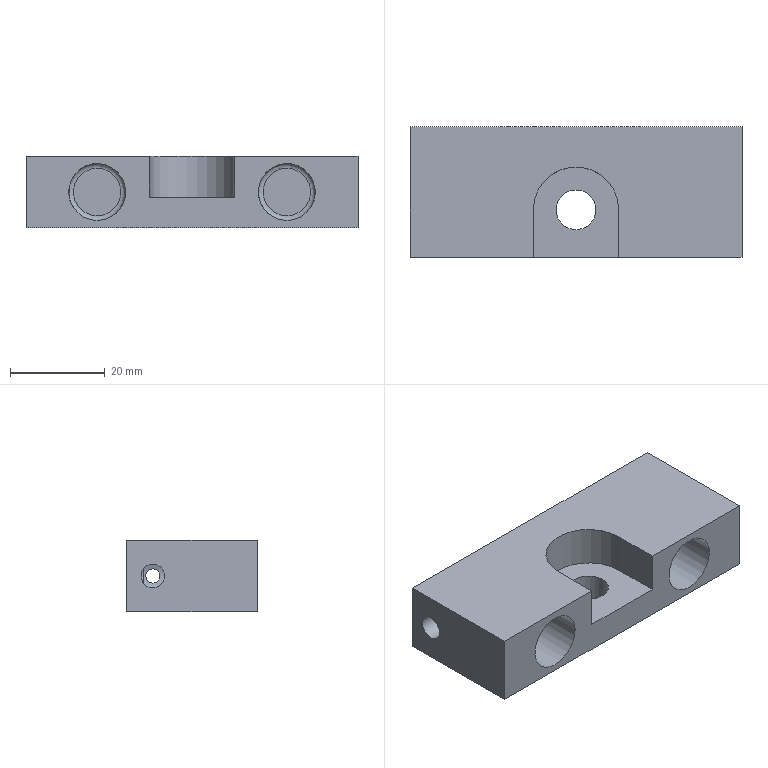NC program | NX | posted with a generic post | part box 70 x 27.5 x 15 mm
Whole program:
N10 G17 G21 G94 G90
(ADAPTIVE_MILLING_1 , TOOL : D10-30-D10-75-3T-ROUGH)
N12 T02 M6
N14 G54
N16 G17 G0 G90 X-47.049 Y-0.548 S3000 M3
N18 G43 Z20. H2
N20 Z3.1
N22 G94 G1 X-46.899 Y-0.555 Z2.163 F1500.
N24 X-46.749 Y-0.561 Z1.792
N26 X-46.599 Y-0.567 Z1.52
N28 X-46.45 Y-0.574 Z1.3
N30 X-46.3 Y-0.58 Z1.116
N32 X-46.15 Y-0.587 Z0.958
N34 X-46. Y-0.593 Z0.82
N36 X-45.85 Y-0.599 Z0.7
N38 X-45.7 Y-0.606 Z0.595
N40 X-45.55 Y-0.612 Z0.502
N42 X-45.401 Y-0.619 Z0.421
N44 X-45.251 Y-0.625 Z0.35
N46 X-45.101 Y-0.631 Z0.29
N48 X-44.951 Y-0.638 Z0.238
N50 X-44.801 Y-0.644 Z0.195
N52 X-44.651 Y-0.65 Z0.161
N54 X-44.501 Y-0.657 Z0.134
N56 X-44.352 Y-0.663 Z0.115
N58 X-44.202 Y-0.67 Z0.104
N60 X-44.052 Y-0.676 Z0.1
N62 X-42.524 Y-0.741
N64 G3 X-41.505 Y0.006 R1.01
N66 X-41.243 Y3.039 R15.515
N68 X-41.191 Y13.418 R760.676
N70 G2 X-38.571 Y17.913 R5.742
N72 X-34.324 Y19.417 R9.801
N74 X-28.522 Y19.69 R46.813
N76 G1 X-23.309 Y19.699
N78 X34.667 Y19.697
N80 G2 X39.423 Y17.065 R5.742
N82 X40.919 Y12.825 R9.795
N84 X41.19 Y6.985 R47.256
N86 G1 X41.2 Y1.473
N88 X41.198 Y-13.179
N90 G2 X38.62 Y-17.874 R5.73
N92 X34.378 Y-19.408 R9.693
N94 X28.877 Y-19.687 R43.278
N96 G1 X22.914 Y-19.699
N98 X-34.605 Y-19.698
N100 G2 X-39.354 Y-17.147 R5.724
N102 X-40.913 Y-12.842 R9.694
N104 X-41.187 Y-7.34 R43.971
N106 X-41.171 Y-1.154 R180.896
N108 G3 X-40.903 Y8.326 R130.717
N110 G2 X-40.865 Y12.33 R70.569
N112 X-37.267 Y17.699 R7.022
N114 X-32.636 Y19.121 R12.052
N116 X-26.307 Y19.39 R57.267
N118 G1 X-20.945 Y19.399
N120 X33.204 Y19.397
N122 G2 X39.157 Y15.843 R6.967
N124 X40.62 Y11.147 R11.956
N126 X40.888 Y5.119 R54.763
N128 G1 X40.899 Y-0.244
N130 G2 X40.883 Y-12.091 R889.062
N132 X37.259 Y-17.701 R7.011
N134 X32.627 Y-19.121 R12.079
N136 X26.374 Y-19.389 R56.687
N138 G1 X20.599 Y-19.399
N140 X-33.217 Y-19.397
N142 G2 X-39.111 Y-15.91 R6.964
N144 X-40.613 Y-11.191 R11.832
N146 X-40.888 Y-5.013 R54.778
N148 X-40.705 Y1.994 R116.295
N150 G3 X-40.584 Y10.798 R488.226
N152 G2 X-36.227 Y17.455 R7.843
N154 X-31.269 Y18.831 R13.871
N156 X-24.264 Y19.091 R70.165
N158 G1 X-20.139 Y19.099
N160 X31.817 Y19.096
N162 G2 X38.958 Y14.725 R7.859
N164 X40.345 Y9.652 R14.018
N166 X40.593 Y2.571 R74.249
N168 X40.583 Y-10.779 R901.961
N170 X36.273 Y-17.428 R7.833
N172 X31.208 Y-18.837 R13.887
N174 X24.053 Y-19.092 R73.09
N176 G1 X19.103 Y-19.099
N178 X-31.792 Y-19.096
N180 G2 X-38.967 Y-14.699 R7.871
N182 X-40.33 Y-9.773 R13.901
N184 X-40.503 Y-0.594 R65.11
N186 G3 X-40.291 Y9.576 R305.228
N188 G2 X-35.334 Y17.191 R8.514
N190 X-30.059 Y18.544 R15.502
N192 X-22.941 Y18.791 R78.806
N194 G1 X-17.578 Y18.799
N196 X30.542 Y18.796
N198 G2 X35.604 Y17.422 R8.994
N200 X39.213 Y12.582 R9.352
N202 X40.156 Y7.168 R20.104
N204 X40.297 Y-0.667 R149.412
N206 X40.273 Y-9.803 R403.654
N208 X35.382 Y-17.165 R8.482
N210 X30.223 Y-18.526 R15.2
N212 X22.955 Y-18.791 R75.544
N214 G1 X17.593 Y-18.799
N216 X-30.48 Y-18.796
N218 G2 X-35.329 Y-17.592 R9.147
N220 X-39.156 Y-12.731 R9.217
N222 X-40.135 Y-7.477 R19.191
N224 X-40.195 Y-0.693 R67.847
N226 G3 X-39.982 Y8.844 R845.986
N228 G2 X-34.546 Y16.909 R9.053
N230 X-29.146 Y18.237 R16.699
N232 X-21.615 Y18.491 R84.996
N234 G1 X-16.253 Y18.498
N236 X29.342 Y18.496
N238 G2 X33.846 Y17.684 R10.9
N240 X38.53 Y12.776 R9.24
N242 X39.772 Y7.276 R17.655
N244 X39.993 Y-0.481 R99.236
N246 X39.97 Y-8.829 R341.491
N248 X34.657 Y-16.853 R9.017
N250 X29.305 Y-18.22 R16.302
N252 X21.7 Y-18.49 R80.981
N254 G1 X16.338 Y-18.498
N256 X-29.354 Y-18.496
N258 G2 X-33.754 Y-17.722 R10.945
N260 X-38.553 Y-12.716 R9.244
N262 X-39.773 Y-7.249 R17.786
N264 X-39.863 Y0.097 R65.603
N266 G1 X-39.688 Y7.961
N268 G2 X-37.744 Y13.614 R9.849
N270 X-32.466 Y17.135 R10.566
N272 X-26.778 Y18.05 R23.313
N274 X-17.106 Y18.197 R190.266
N276 G1 X27.879
N278 G2 X32.043 Y17.769 R15.077
N280 X38.037 Y12.505 R9.415
N282 X39.417 Y6.962 R17.239
N284 X39.689 Y-0.568 R82.563
N286 X39.66 Y-8.067 R208.183
N288 X37.304 Y-14.13 R9.6
N290 X32.016 Y-17.268 R10.993
N292 X26.31 Y-18.075 R25.674
N294 X15.25 Y-18.198 R262.965
N296 G1 X-28.192 Y-18.196
N298 G2 X-32.52 Y-17.62 R13.255
N300 X-38.027 Y-12.521 R9.447
N302 X-39.406 Y-7.015 R17.006
N304 X-39.556 Y-0.009 R58.525
N306 X-39.388 Y7.263 R563.307
N308 X-37.613 Y12.797 R10.513
N310 X-32.256 Y16.675 R10.651
N312 X-26.591 Y17.705 R22.061
N314 X-18.007 Y17.895 R135.745
N316 G1 X-13.882 Y17.898
N318 X27.129 Y17.896
N320 G2 X31.405 Y17.449 R15.965
N322 X37.649 Y12.042 R9.738
N324 X39.077 Y6.512 R17.412
N326 X39.387 Y-1.316 R78.81
N328 X39.346 Y-7.428 R123.509
N330 X37.205 Y-13.322 R10.135
N332 X31.856 Y-16.804 R10.986
N334 X26.019 Y-17.742 R24.168
N336 X16.234 Y-17.897 R188.951
N338 G1 X-26.729
N340 G2 X-30.871 Y-17.581 R19.053
N342 X-37.64 Y-12.055 R9.726
N344 X-39.083 Y-6.333 R17.262
N346 X-39.236 Y0.524 R60.889
N348 X-39.076 Y6.782 R166.058
N350 X-37.176 Y12.432 R10.843
N352 X-31.715 Y16.338 R11.001
N354 X-25.79 Y17.405 R22.957
N356 X-16.944 Y17.594 R143.25
N358 G1 X-12.819 Y17.598
N360 X26.079 Y17.596
N362 G2 X30.441 Y17.223 R19.062
N364 X37.312 Y11.506 R10.047
N366 X38.772 Y5.789 R18.081
N368 X39.087 Y-2.264 R82.195
N370 X38.992 Y-7.286 R54.073
N372 X32.842 Y-15.885 R10.138
N374 X27.145 Y-17.286 R18.516
N376 X19.016 Y-17.587 R86.411
N378 G1 X12.829 Y-17.597
N380 X-26.092 Y-17.596
N382 G2 X-30.416 Y-17.228 R19.058
N384 X-37.318 Y-11.488 R10.055
N386 X-38.775 Y-5.501 R17.921
N388 X-38.906 Y1.882 R72.646
N390 X-38.718 Y6.751 R55.237
N392 X-35.588 Y13.398 R10.569
N394 X-29.966 Y16.376 R12.56
N396 X-23.729 Y17.177 R30.37
N398 X-12.106 Y17.297 R304.578
N400 G1 X25.254 Y17.296
N402 G2 X29.767 Y16.928 R20.792
N404 X36.951 Y11.05 R10.325
N406 X38.462 Y5.154 R18.548
N408 X38.784 Y-2.824 R81.692
N410 X38.578 Y-7.464 R29.494
N412 X32.446 Y-15.497 R10.365
N414 X26.538 Y-16.973 R18.858
N416 X18.56 Y-17.284 R84.336
N418 G1 X12.372 Y-17.297
N420 X-25.267 Y-17.295
N422 G2 X-29.853 Y-16.907 R20.376
N424 X-36.998 Y-10.939 R10.339
N426 X-38.443 Y-4.95 R18.282
N428 X-38.59 Y2.546 R75.16
N430 X-38.236 Y7.326 R27.053
N432 X-31.991 Y15.155 R10.681
N434 X-26.125 Y16.644 R19.116
N436 X-18.486 Y16.978 R77.685
N438 G1 X-11.473 Y16.997
N440 X24.317 Y16.995
N442 G2 X29.021 Y16.652 R23.524
N444 X36.612 Y10.569 R10.591
N446 X38.141 Y4.64 R18.898
N448 X38.402 Y-5.66 R72.389
N450 X36.42 Y-11.56 R11.403
N452 X30.843 Y-15.615 R11.444
N454 X24.671 Y-16.777 R23.416
N456 X15.6 Y-16.993 R136.347
N458 G1 X11.475 Y-16.997
N460 X-24.329 Y-16.995
N462 G2 X-28.923 Y-16.671 R23.893
N464 X-36.63 Y-10.517 R10.584
N466 X-38.112 Y-4.422 R18.517
N468 X-38.145 Y5.281 R66.546
N470 X-35.972 Y11.306 R11.757
N472 X-30.227 Y15.339 R11.851
N474 X-24.122 Y16.467 R24.249
N476 X-14.864 Y16.692 R136.85
N478 G1 X-10.739 Y16.697
N480 X23.679 Y16.694
N482 G2 X28.531 Y16.327 R24.071
N484 X36.265 Y10.124 R10.83
N486 X37.833 Y4.051 R19.314
N488 X38.083 Y-5.124 R59.586
N490 X36.044 Y-11.158 R11.684
N492 X30.348 Y-15.288 R11.686
N494 X24.176 Y-16.462 R23.767
N496 X14.693 Y-16.693 R136.509
N498 G1 X10.568 Y-16.697
N500 X-23.692 Y-16.694
N502 G2 X-28.434 Y-16.346 R24.451
N504 X-36.319 Y-9.985 R10.822
N506 X-37.77 Y-4.037 R18.785
N508 X-37.82 Y4.914 R52.811
N510 X-35.456 Y11.108 R11.843
N512 X-29.66 Y15.044 R12.192
N514 X-23.44 Y16.169 R25.15
N516 X-14.37 Y16.391 R137.551
N518 G1 X-9.42 Y16.396
N520 X22.742 Y16.395
N522 G2 X27.711 Y16.072 R27.77
N524 X36.008 Y9.503 R11.102
N526 X37.52 Y3.524 R19.933
N528 X37.749 Y-4.75 R48.245
N530 X35.489 Y-11.012 R11.747
N532 X29.651 Y-15.038 R12.091
N534 X23.507 Y-16.162 R24.895
N536 X14.286 Y-16.391 R135.773
N538 G1 X9.336 Y-16.396
N540 X-22.829 Y-16.394
N542 G2 X-27.761 Y-16.062 R27.034
N544 X-36.002 Y-9.478 R11.047
N546 X-37.461 Y-3.339 R19.434
N548 X-37.492 Y4.525 R43.189
N550 X-34.954 Y10.895 R11.944
N552 X-28.963 Y14.797 R12.587
N554 X-22.546 Y15.886 R26.879
N556 X-13.437 Y16.091 R151.83
N558 G1 X-9.312 Y16.096
N560 X21.804 Y16.095
N562 G2 X26.928 Y15.807 R32.06
N564 X35.66 Y9.093 R11.32
N566 X37.204 Y3.046 R20.158
N568 X37.396 Y-4.515 R38.871
N570 X34.69 Y-11.152 R11.638
N572 X28.806 Y-14.838 R12.676
N574 X22.495 Y-15.888 R27.197
N576 X13.424 Y-16.091 R152.342
N578 G1 X9.299 Y-16.096
N580 X-21.892 Y-16.095
N582 G2 X-26.94 Y-15.805 R31.463
N584 X-35.715 Y-8.918 R11.278
N586 X-37.149 Y-2.696 R20.144
N588 X-37.135 Y4.342 R34.667
N590 X-33.948 Y11.233 R11.777
N592 X-27.928 Y14.651 R13.419
N594 X-21.226 Y15.628 R30.675
N596 X-9.753 Y15.795 R237.803
N598 G1 X20.454
N600 G2 X25.958 Y15.567 R42.075
N602 X32.904 Y12.242 R11.703
N604 X36.196 Y6.248 R13.557
N606 X37.151 Y-1.212 R31.544
N608 X36.548 Y-6.705 R17.579
N610 X30.328 Y-13.745 R11.358
N612 X24.263 Y-15.365 R19.911
N614 X16.252 Y-15.769 R74.044
N616 G1 X7.964 Y-15.796
N618 X-21.329 Y-15.794
N620 G2 X-26.452 Y-15.491 R31.867
N622 X-35.4 Y-8.43 R11.467
N624 X-36.825 Y-2.203 R20.52
N626 X-36.728 Y4.417 R27.619
N628 X-29.744 Y13.507 R11.71
N630 X-23.517 Y15.089 R20.934
N632 X-15.43 Y15.471 R80.018
N634 G1 X-7.592 Y15.496
N636 X20.604 Y15.494
N638 G2 X25.84 Y15.201 R34.266
N640 X35.047 Y8.128 R11.734
N642 X36.624 Y1.665 R21.325
N644 X36.598 Y-4.544 R24.59
N646 X29.941 Y-13.396 R11.513
N648 X23.811 Y-15.049 R20.104
N650 X15.426 Y-15.471 R75.925
N652 G1 X7.589 Y-15.495
N654 X-20.474 Y-15.494
N656 G2 X-25.897 Y-15.191 R34.577
N658 X-35.024 Y-8.095 R11.63
N660 X-36.514 Y-1.538 R20.763
N662 X-36.274 Y4.624 R22.165
N664 X-29.497 Y13.1 R11.773
N666 X-23.211 Y14.758 R20.739
N668 X-14.938 Y15.169 R78.01
N670 G1 X-6.275 Y15.195
N672 X19.725 Y15.194
N674 G2 X25.225 Y14.912 R37.881
N676 X32.455 Y11.213 R11.987
N678 X35.625 Y5.1 R14.282
N680 X36.318 Y-3.603 R25.05
N682 X29.4 Y-13.123 R11.673
N684 X23.113 Y-14.766 R20.789
N686 X14.539 Y-15.172 R81.141
N688 G1 X6.289 Y-15.195
N690 X-19.867 Y-15.193
N692 G2 X-25.328 Y-14.896 R36.103
N694 X-32.581 Y-11.05 R11.856
N696 X-35.589 Y-4.949 R14.173
N698 X-36.037 Y3.615 R23.069
N700 X-29.172 Y12.732 R11.875
N702 X-22.936 Y14.424 R20.596
N704 X-14.552 Y14.865 R75.07
N706 G1 X-5.89 Y14.895
N708 X19.141 Y14.893
N710 G2 X24.717 Y14.608 R38.933
N712 X31.806 Y11.156 R12.251
N714 X35.24 Y4.907 R14.108
N716 X35.924 Y-3.453 R22.127
N718 X29.228 Y-12.679 R11.688
N720 X22.927 Y-14.42 R20.312
N722 X14.544 Y-14.865 R74.343
N724 G1 X5.881 Y-14.895
N726 X-18.956 Y-14.894
N728 G2 X-24.57 Y-14.629 R41.378
N730 X-31.347 Y-11.581 R12.343
N732 X-35.05 Y-5.312 R13.404
N734 X-35.64 Y3.452 R20.621
N736 X-28.786 Y12.396 R11.928
N738 X-22.405 Y14.123 R20.888
N740 X-14.059 Y14.563 R76.012
N742 G1 X-6.184 Y14.595
N744 X18.316 Y14.593
N746 G2 X24.006 Y14.335 R43.661
N748 X30.714 Y11.483 R12.73
N750 X34.684 Y5.268 R13.48
N752 X35.504 Y-3.397 R19.743
N754 X28.991 Y-12.266 R11.693
N756 X22.746 Y-14.072 R19.932
N758 X14.366 Y-14.559 R69.645
N760 G1 X5.666 Y-14.595
N762 X-18.404 Y-14.593
N764 G2 X-24.13 Y-14.317 R41.848
N766 X-30.831 Y-11.362 R12.542
N768 X-34.641 Y-5.157 R13.336
N770 X-35.23 Y3.299 R18.608
N772 X-28.604 Y11.963 R11.915
N774 X-22.096 Y13.795 R20.603
N776 X-13.563 Y14.262 R74.647
N778 G1 X-4.488 Y14.295
N780 X17.754 Y14.293
N782 G2 X23.667 Y14.01 R43.357
N784 X30.459 Y11.043 R12.828
N786 X34.375 Y4.812 R13.652
N788 X35.07 Y-3.336 R17.768
N790 X28.629 Y-11.916 R11.705
N792 X22.428 Y-13.743 R19.896
N794 X14.312 Y-14.25 R66.012
N796 X4.412 Y-14.294 R695.89
N798 G1 X-17.613 Y-14.293
N800 G2 X-23.491 Y-14.035 R45.945
N802 X-29.986 Y-11.417 R12.973
N804 X-34.211 Y-5.055 R13.114
N806 X-34.775 Y3.313 R16.858
N808 X-28.301 Y11.589 R11.899
N810 X-22.029 Y13.434 R20.176
N812 X-13.763 Y13.95 R67.034
N814 X-3.863 Y13.994 R696.051
N816 G1 X16.924 Y13.993
N818 G2 X22.915 Y13.744 R49.126
N820 X29.396 Y11.268 R13.429
N822 X33.92 Y4.797 R13.295
N824 X34.623 Y-3.262 R16.209
N826 X28.472 Y-11.461 R11.648
N828 X22.154 Y-13.407 R19.525
N830 X14.115 Y-13.943 R63.11
N832 X3.803 Y-13.994 R696.807
N834 G1 X-17.054 Y-13.993
N836 G2 X-23.044 Y-13.726 R46.616
N838 X-29.557 Y-11.123 R13.167
N840 X-33.948 Y-4.406 R13.208
N842 X-34.235 Y3.593 R15.163
N844 X-28.116 Y11.153 R11.85
N846 X-21.796 Y13.094 R19.803
N848 X-13.683 Y13.641 R63.406
N850 X-2.958 Y13.694 R708.916
N852 G1 X16.367 Y13.693
N854 G2 X22.432 Y13.441 R50.383
N856 X28.992 Y10.96 R13.661
N858 X33.669 Y4.15 R13.372
N860 X34.091 Y-3.51 R14.607
N862 X28.095 Y-11.121 R11.628
N864 X21.71 Y-13.098 R19.616
N866 X13.671 Y-13.64 R63.163
N868 X3.359 Y-13.694 R694.361
N870 G1 X-16.266 Y-13.693
N872 G2 X-22.37 Y-13.449 R51.85
N874 X-28.694 Y-11.153 R13.685
N876 X-33.518 Y-4.284 R12.955
N878 X-33.676 Y3.809 R13.925
N880 X-27.76 Y10.808 R11.832
N882 X-21.302 Y12.794 R19.949
N884 X-13.076 Y13.341 R64.774
N886 X-2.351 Y13.394 R710.856
N888 G1 X15.624 Y13.393
N890 G2 X21.953 Y13.14 R53.29
N892 X28.466 Y10.744 R13.932
N894 X33.417 Y3.446 R13.321
N896 X33.349 Y-4.31 R13.079
N898 X27.624 Y-10.831 R11.678
N900 X21.347 Y-12.777 R19.685
N902 X13.384 Y-13.334 R61.734
N904 X2.247 Y-13.394 R711.438
N906 G1 X-15.704 Y-13.392
N908 G2 X-21.921 Y-13.143 R52.73
N910 X-28.31 Y-10.83 R13.87
N912 X-33.326 Y-3.291 R12.967
N914 X-32.733 Y4.895 R12.501
N916 X-26.966 Y10.688 R12.059
N918 X-20.43 Y12.549 R21.063
N920 X-11.713 Y13.054 R73.957
N922 X-1.813 Y13.093 R710.126
N924 G1 X15.337 Y13.092
N926 G2 X21.664 Y12.814 R50.499
N928 X28.223 Y10.325 R13.942
N930 X33.352 Y1.631 R13.297
N932 X30.794 Y-7.698 R11.376
N934 X24.846 Y-11.53 R13.54
N936 X17.894 Y-12.811 R28.404
N938 X7.25 Y-13.087 R151.471
N940 G1 X1.888 Y-13.093
N942 X-15.375 Y-13.092
N944 G2 X-21.664 Y-12.813 R49.863
N946 X-28.179 Y-10.328 R13.794
N948 X-32.974 Y2.587 R12.825
N950 X-27.41 Y9.909 R11.505
N952 X-20.975 Y12.091 R18.941
N954 X-12.831 Y12.723 R57.793
N956 X-1.282 Y12.793 R689.358
N958 G1 X14.792 Y12.791
N960 G2 X21.194 Y12.514 R51.806
N962 X27.78 Y10.055 R14.174
N964 X32.885 Y-1.973 R12.714
N966 X27.527 Y-9.772 R11.185
N968 X21.24 Y-12.031 R18.126
N970 X13.552 Y-12.703 R51.848
N972 X1.402 Y-12.793 R517.989
N974 G1 X-14.804 Y-12.791
N976 G2 X-21.057 Y-12.53 R52.855
N978 X-27.432 Y-10.268 R14.238
N980 X-32.557 Y2.087 R12.246
N982 X-27.356 Y9.372 R11.267
N984 X-21.055 Y11.692 R18.059
N986 X-13.482 Y12.39 R50.097
N988 X-0.695 Y12.493 R477.475
N990 G1 X14.13 Y12.491
N992 G2 X20.608 Y12.228 R55.433
N994 X27.073 Y9.968 R14.599
N996 X32.467 Y-1.159 R12.197
N998 X27.562 Y-9.157 R10.904
N1000 X21.387 Y-11.608 R17.1
N1002 X13.822 Y-12.376 R46.025
N1004 X0.998 Y-12.493 R419.773
N1006 G1 X-14.165 Y-12.491
N1008 G2 X-20.68 Y-12.217 R54.019
N1010 X-27.141 Y-9.888 R14.298
N1012 X-32.176 Y1.175 R11.769
N1014 X-27.259 Y8.845 R10.973
N1016 X-21.035 Y11.303 R17.319
N1018 X-13.32 Y12.078 R46.968
N1020 X-0.271 Y12.193 R438.043
N1022 G1 X13.554 Y12.191
N1024 G2 X20.108 Y11.933 R57.674
N1026 X26.554 Y9.747 R14.894
N1028 X31.994 Y-0.129 R11.771
N1030 X27.456 Y-8.611 R10.608
N1032 X21.34 Y-11.216 R16.42
N1034 X13.785 Y-12.058 R42.888
N1036 X0.511 Y-12.192 R379.68
N1038 G1 X-13.564 Y-12.191
N1040 G2 X-20.08 Y-11.934 R57.505
N1042 X-26.394 Y-9.816 R14.76
N1044 X-31.732 Y-0.036 R11.381
N1046 X-27.266 Y8.22 R10.607
N1048 X-21.103 Y10.886 R16.403
N1050 X-13.512 Y11.751 R42.55
N1052 X0.586 Y11.892 R388.54
N1054 G1 X12.992 Y11.891
N1056 G2 X19.695 Y11.627 R58.83
N1058 X25.986 Y9.554 R15.12
N1060 X31.415 Y0.955 R11.404
N1062 X27.438 Y-7.97 R10.26
N1064 X21.428 Y-10.783 R15.536
N1066 X14.224 Y-11.714 R38.082
N1068 X2.414 Y-11.891 R261.192
N1070 G1 X-11.767 Y-11.892
N1072 G2 X-18.85 Y-11.714 R85.425
N1074 X-24.875 Y-10.148 R16.516
N1076 X-31.034 Y-2.115 R11.249
N1078 X-27.552 Y7.318 R10.135
N1080 X-21.573 Y10.353 R15.
N1082 X-14.457 Y11.378 R35.229
N1084 X-3.435 Y11.588 R208.471
N1086 G1 X1.102 Y11.592
N1088 X12.429 Y11.591
N1090 G2 X19.096 Y11.344 R62.584
N1092 X25.388 Y9.375 R15.531
N1094 X30.739 Y1.869 R11.073
N1096 X27.4 Y-7.301 R9.904
N1098 X21.507 Y-10.337 R14.691
N1100 X14.358 Y-11.379 R34.686
N1102 X3.524 Y-11.588 R205.014
N1104 G1 X-0.601 Y-11.592
N1106 X-12.389 Y-11.591
N1108 G2 X-19.168 Y-11.333 R61.284
N1110 X-25.37 Y-9.347 R15.174
N1112 X-30.486 Y-1.978 R10.682
N1114 X-27.222 Y6.887 R9.842
N1116 X-21.411 Y9.966 R14.548
N1118 X-14.458 Y11.047 R33.149
N1120 X-2.837 Y11.288 R195.121
N1122 G1 X1.7 Y11.292
N1124 G2 X15.438 Y11.249 R825.109
N1126 X21.421 Y10.541 R26.583
N1128 X28.017 Y6.484 R12.44
N1130 X29.557 Y-3.351 R9.564
N1132 X24.62 Y-8.607 R10.959
N1134 X18.472 Y-10.594 R19.225
N1136 X10.327 Y-11.217 R59.571
N1138 X-1.223 Y-11.292 R665.103
N1140 X-15.447 Y-11.249 R847.179
N1142 X-21.283 Y-10.567 R26.492
N1144 X-27.645 Y-6.779 R12.23
N1146 X-27.224 Y6.105 R9.415
N1148 X-21.492 Y9.497 R13.647
N1150 X-14.599 Y10.702 R30.215
N1152 X-3.805 Y10.984 R157.84
N1154 G1 X1.557 Y10.991
N1156 G2 X15.182 Y10.942 R688.484
N1158 X21.195 Y10.189 R25.893
N1160 X27.455 Y6.346 R12.198
N1162 X27.052 Y-6.063 R9.197
N1164 X21.388 Y-9.483 R13.327
N1166 X14.61 Y-10.693 R29.441
N1168 X4.791 Y-10.98 R140.944
N1170 G1 X-1.809 Y-10.991
N1172 G2 X-14.946 Y-10.949 R681.525
N1174 X-20.929 Y-10.248 R26.811
N1176 X-26.957 Y-6.763 R12.08
N1178 X-26.928 Y5.565 R9.063
N1180 X-21.337 Y9.088 R13.079
N1182 X-14.499 Y10.37 R28.473
N1184 X-4.419 Y10.679 R136.71
N1186 G1 X2.181 Y10.691
N1188 G2 X14.644 Y10.644 R577.374
N1190 X20.662 Y9.92 R26.824
N1192 X26.608 Y6.509 R12.143
N1194 X26.743 Y-5.513 R8.862
N1196 X21.336 Y-9.031 R12.682
N1198 X14.619 Y-10.35 R27.208
N1200 X4.54 Y-10.678 R128.587
N1202 G1 X-2.06 Y-10.691
N1204 G2 X-14.672 Y-10.642 R639.241
N1206 X-20.579 Y-9.929 R26.413
N1208 X-26.345 Y-6.636 R11.81
N1210 X-26.63 Y4.979 R8.715
N1212 X-21.206 Y8.659 R12.454
N1214 X-14.688 Y10.009 R26.197
N1216 X-4.985 Y10.372 R114.237
N1218 G1 X2.44 Y10.391
N1220 G2 X14.489 Y10.333 R501.017
N1222 X20.428 Y9.572 R25.827
N1224 X26.052 Y6.318 R11.742
N1226 X26.348 Y-5.015 R8.535
N1228 X21.026 Y-8.659 R12.216
N1230 X14.396 Y-10.025 R26.028
N1232 X4.58 Y-10.374 R118.632
N1234 G1 X-2.845 Y-10.391
N1236 G2 X-14.519 Y-10.331 R467.322
N1238 X-20.49 Y-9.538 R24.954
N1240 X-25.856 Y-6.35 R11.241
N1242 X-26.234 Y4.453 R8.385
N1244 X-20.992 Y8.246 R11.901
N1246 X-14.418 Y9.687 R24.882
N1248 X-4.492 Y10.072 R110.817
N1250 X13.595 Y10.046 R935.861
N1252 X19.657 Y9.365 R28.447
N1254 X25.028 Y6.579 R11.84
N1256 X25.875 Y-4.564 R8.235
N1258 X20.785 Y-8.249 R11.703
N1260 X14.436 Y-9.67 R24.174
N1262 X5.035 Y-10.066 R101.802
N1264 X-13.352 Y-10.052 R959.148
N1266 X-19.346 Y-9.426 R29.509
N1268 X-24.606 Y-6.816 R11.66
N1270 X-25.68 Y4.083 R8.095
N1272 X-20.615 Y7.884 R11.476
N1274 X-14.387 Y9.336 R23.449
N1276 X-5.476 Y9.757 R92.19
N1278 X13.211 Y9.744 R833.609
N1280 X19.2 Y9.075 R28.592
N1282 X24.334 Y6.471 R11.474
N1284 X25.372 Y-4.098 R7.934
N1286 X20.344 Y-7.906 R11.266
N1288 X14.079 Y-9.354 R23.296
N1290 X4.604 Y-9.765 R98.764
N1292 X-13.22 Y-9.743 R815.285
N1294 X-19.17 Y-9.065 R27.804
N1296 X-24.14 Y-6.476 R10.909
N1298 X-25.169 Y3.595 R7.792
N1300 X-20.232 Y7.512 R10.98
N1302 X-13.947 Y9.028 R22.554
N1304 X-5.036 Y9.456 R90.597
N1306 X12.976 Y9.437 R708.338
N1308 X18.85 Y8.757 R27.886
N1310 X23.739 Y6.242 R10.85
N1312 X24.786 Y-3.684 R7.648
N1314 X20.048 Y-7.488 R10.741
N1316 X13.916 Y-9.012 R21.743
N1318 X5.043 Y-9.455 R86.626
N1320 X-12.706 Y-9.444 R771.253
N1322 X-18.622 Y-8.794 R28.429
N1324 X-23.332 Y-6.425 R10.526
N1326 X-24.567 Y3.166 R7.511
N1328 X-19.806 Y7.144 R10.511
N1330 X-13.722 Y8.693 R21.268
N1332 X-4.739 Y9.153 R84.98
N1334 X12.586 Y9.135 R638.049
N1336 X18.495 Y8.438 R27.386
N1338 X23.071 Y6.047 R10.149
N1340 X24.15 Y-3.275 R7.378
N1342 X19.498 Y-7.164 R10.335
N1344 X13.451 Y-8.703 R20.97
N1346 X4.542 Y-9.155 R84.863
N1348 X-12.27 Y-9.143 R712.641
N1350 X-18.077 Y-8.52 R28.706
N1352 X-22.623 Y-6.246 R9.952
N1354 X-23.878 Y2.797 R7.245
N1356 X-19.3 Y6.794 R10.085
N1358 X-13.299 Y8.378 R20.33
N1360 X-4.616 Y8.848 R80.125
N1362 X12.183 Y8.833 R581.753
N1364 X17.874 Y8.185 R27.742
N1366 X22.299 Y5.911 R9.595
N1368 X23.435 Y-2.908 R7.121
N1370 X18.975 Y-6.81 R9.91
N1372 X13.277 Y-8.353 R19.572
N1374 X4.633 Y-8.846 R75.381
N1376 X-12.166 Y-8.832 R569.212
N1378 X-17.744 Y-8.191 R26.711
N1380 X-22.049 Y-5.891 R9.01
N1382 X-23.071 Y2.543 R7.008
N1384 X-18.684 Y6.474 R9.727
N1386 X-12.956 Y8.048 R19.238
N1388 X-4.351 Y8.544 R74.914
N1390 X11.774 Y8.532 R528.659
N1392 X17.39 Y7.893 R27.238
N1394 X21.609 Y5.648 R8.794
N1396 X22.663 Y-2.54 R6.877
N1398 X18.249 Y-6.53 R9.553
N1400 X12.474 Y-8.082 R19.248
N1402 X3.979 Y-8.547 R77.101
N1404 X-11.695 Y-8.533 R526.196
N1406 X-17.199 Y-7.909 R26.319
N1408 X-21.374 Y-5.565 R8.227
N1410 X-22.22 Y2.27 R6.783
N1412 X-17.906 Y6.211 R9.417
N1414 X-12.325 Y7.753 R18.66
N1416 X-4.019 Y8.241 R72.205
N1418 X11.543 Y8.224 R452.237
N1420 X16.86 Y7.607 R25.804
N1422 X20.993 Y5.226 R7.906
N1424 X21.681 Y-2.449 R6.687
N1426 X17.371 Y-6.3 R9.345
N1428 X11.621 Y-7.812 R19.068
N1430 X2.974 Y-8.253 R81.091
N1432 X-11.351 Y-8.229 R466.236
N1434 X-16.486 Y-7.663 R25.759
N1436 X-20.615 Y-5.245 R7.544
N1438 X-21.209 Y2.177 R6.596
N1440 X-16.887 Y6.037 R9.241
N1442 X-11.36 Y7.498 R18.744
N1444 X-2.939 Y7.949 R77.303
N1446 X11.085 Y7.925 R416.054
N1448 X16.217 Y7.34 R24.872
N1450 X20.34 Y4.714 R7.126
N1452 X20.622 Y-2.374 R6.522
N1454 X16.324 Y-6.122 R9.179
N1456 X10.78 Y-7.536 R18.906
N1458 X2.432 Y-7.953 R80.893
N1460 X-11.143 Y-7.921 R389.9
N1462 X-15.83 Y-7.392 R23.557
N1464 X-20.111 Y-4.413 R6.746
N1466 X-19.946 Y2.391 R6.503
N1468 X-15.554 Y5.971 R9.319
N1470 X-9.947 Y7.287 R19.91
N1472 X-1.071 Y7.664 R94.266
N1474 X11.115 Y7.606 R310.034
N1476 X15.573 Y7.06 R21.277
N1478 X19.966 Y3.36 R6.345
N1480 X18.963 Y-3.085 R6.585
N1482 X14.432 Y-6.254 R9.778
N1484 X8.595 Y-7.39 R22.704
N1486 X-0.886 Y-7.676 R128.101
N1488 X-11.385 Y-7.591 R236.562
N1490 X-15.388 Y-7.042 R17.372
N1492 X-19.367 Y1.128 R6.049
N1494 X-15.427 Y5.308 R8.254
N1496 X-10.13 Y6.874 R16.117
N1498 X-2.199 Y7.342 R66.632
N1500 X10.813 Y7.3 R285.029
N1502 X14.785 Y6.797 R18.062
N1504 X18.793 Y-1.088 R5.924
N1506 X14.957 Y-5.302 R8.04
N1508 X9.923 Y-6.85 R15.295
N1510 X2.331 Y-7.336 R60.01
N1512 X-10.755 Y-7.299 R276.317
N1514 X-14.354 Y-6.832 R15.711
N1516 X-18.245 Y0.626 R5.788
N1518 X-14.642 Y4.884 R7.766
N1520 X-9.523 Y6.542 R14.532
N1522 X-2.27 Y7.03 R56.483
N1524 X10.366 Y7. R258.581
N1526 X13.745 Y6.575 R15.136
N1528 X17.621 Y-0.513 R5.654
N1530 X14.187 Y-4.827 R7.526
N1532 X9.209 Y-6.524 R13.721
N1534 X2.22 Y-7.025 R51.637
N1536 X-10.266 Y-7. R248.591
N1538 X-13.376 Y-6.565 R11.858
N1540 X-16.966 Y0.117 R5.527
N1542 X-13.517 Y4.575 R7.376
N1544 X-8.61 Y6.24 R13.506
N1546 X-1.507 Y6.731 R52.524
N1548 X10.116 Y6.689 R212.404
N1550 X13.022 Y6.192 R9.003
N1552 X16.222 Y-0.128 R5.409
N1554 X12.845 Y-4.601 R7.222
N1556 X8.049 Y-6.25 R13.094
N1558 X1.471 Y-6.725 R48.73
N1560 X-9.965 Y-6.69 R200.689
N1562 X-13.087 Y-5.871 R6.382
N1564 X-15.375 Y0.141 R5.357
N1566 X-11.992 Y4.411 R7.198
N1568 X-7.066 Y6.015 R13.315
N1570 X-0.072 Y6.443 R55.904
N1572 X9.751 Y6.377 R159.667
N1574 X14.642 Y0.438 R5.129
N1576 X11.627 Y-4.175 R6.787
N1578 X6.882 Y-5.949 R11.905
N1580 X0.381 Y-6.431 R44.95
N1582 X-9.217 Y-6.394 R159.39
N1584 X-13.773 Y-1.166 R4.941
N1586 X-11.111 Y3.67 R6.48
N1588 X-6.588 Y5.577 R10.853
N1590 X-0.656 Y6.111 R36.238
N1592 X8.53 Y6.1 R134.544
N1594 X12.759 Y1.298 R4.779
N1596 X10.3 Y-3.608 R6.28
N1598 X5.725 Y-5.599 R10.428
N1600 X0.055 Y-6.113 R34.596
N1602 X-7.519 Y-6.131 R158.766
N1604 X-11.65 Y-1.792 R4.598
N1606 X-9.503 Y3.153 R6.056
N1608 X-5.106 Y5.25 R9.714
N1610 X0.596 Y5.813 R30.934
N1612 X6.482 Y5.84 R142.497
N1614 X10.377 Y2.018 R4.4
N1616 X8.542 Y-3.008 R5.833
N1618 X4.286 Y-5.212 R9.111
N1620 X-0.959 Y-5.801 R26.39
N1622 X-5.383 Y-5.837 R62.464
N1624 X-8.955 Y-2.461 R4.189
N1626 X-7.388 Y2.597 R5.64
N1628 X-3.124 Y4.919 R8.721
N1630 X1.934 Y5.501 R24.641
N1632 X4.181 Y5.499 R15.401
N1634 X7.324 Y2.48 R3.976
N1636 X5.958 Y-2.533 R5.474
N1638 X1.745 Y-4.926 R8.38
N1640 X-2.262 Y-5.438 R16.973
N1642 X-4.795 Y-3.868 R3.554
N1644 X-4.568 Y2.148 R5.052
N1646 X-1.352 Y4.395 R7.118
N1648 G1 X-0.936 Y4.566
N1650 X-0.799 Y4.628 Z0.104
N1652 X-0.662 Y4.69 Z0.115
N1654 X-0.526 Y4.751 Z0.134
N1656 X-0.389 Y4.813 Z0.161
N1658 X-0.252 Y4.875 Z0.195
N1660 X-0.116 Y4.937 Z0.238
N1662 X0.021 Y4.999 Z0.29
N1664 X0.158 Y5.06 Z0.35
N1666 X0.294 Y5.122 Z0.421
N1668 X0.431 Y5.184 Z0.502
N1670 X0.568 Y5.246 Z0.595
N1672 X0.705 Y5.307 Z0.7
N1674 X0.841 Y5.369 Z0.82
N1676 X0.978 Y5.431 Z0.958
N1678 X1.115 Y5.493 Z1.116
N1680 X1.251 Y5.554 Z1.3
N1682 X1.388 Y5.616 Z1.52
N1684 X1.525 Y5.678 Z1.792
N1686 X1.661 Y5.74 Z2.163
N1688 X1.798 Y5.801 Z3.1
N1690 G0 Z20.
N1692 M5
(PLANAR_MILL_5 , TOOL : D50面刀)
N1694 T01 M6
N1696 G54
N1698 G17 G0 G90 X65. Y-0.05 S1600 M3
N1700 G43 Z20. H1
N1702 Z3.
N1704 G94 G1 Z0. F800.
N1706 X35.
N1708 X-35.
N1710 X-65.
N1712 Z3.
N1714 G0 Z20.
N1716 M5
(PLANAR_MILL_7 , TOOL : 倒角D4-90度)
N1718 T05 M6
N1720 G54
N1722 G17 G0 G90 X1.625 Y-4.25 S3000 M3
N1724 G43 Z20. H5
N1726 Z0.
N1728 G94 G1 Z-2. F800.
N1730 X1.7
N1732 G3 X2.2 Y-3.75 R0.5
N1734 X0. Y-1.55 R2.2
N1736 X2.2 Y-3.75 R-2.2
N1738 X1.7 Y-3.25 R0.5
N1740 G1 X1.625
N1742 Z0.
N1744 G0 Z20.
(PLANAR_MILL_6 , TOOL : 倒角D4-90度)
N1746 X38.464 Y-15.75
N1748 Z1.
N1750 G1 Z-2.
N1752 X34.999
N1754 X-35.
N1756 G2 X-37. Y-13.75 R2.
N1758 G1 Y13.75
N1760 G2 X-35. Y15.75 R2.
N1762 G1 X35.
N1764 G2 X37. Y13.75 R2.
N1766 G1 Y-13.749
N1768 Y-17.214
N1770 Z1.
N1772 G0 Z20.
N1774 M5
N1776 M2